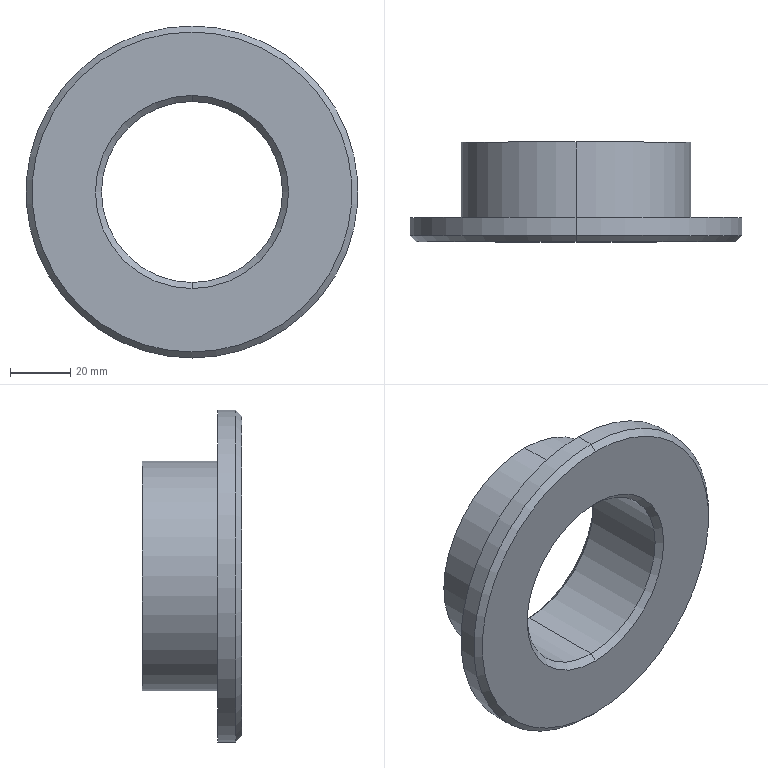Part | SolidWorks | features Chamfer 1, Revolution 1 | 1 solid | 15 faces | box 110 x 33 x 110 mm | volume 94679 mm3 | cone 6 | cylinder 6 | plane 3 | commonest cylinder face diameters 60 x2 76 x2 110 x2
STEP:
#1=CARTESIAN_POINT('',(0.,2.,30.));
#2=VERTEX_POINT('',#1);
#3=CARTESIAN_POINT('',(0.,2.,-30.));
#4=VERTEX_POINT('',#3);
#5=CARTESIAN_POINT('',(0.,2.,0.));
#6=DIRECTION('',(0.,-1.,0.));
#7=DIRECTION('',(0.,0.,1.));
#8=AXIS2_PLACEMENT_3D('',#5,#6,#7);
#9=CIRCLE('',#8,30.);
#10=EDGE_CURVE('',#2,#4,#9,.T.);
#11=ORIENTED_EDGE('',*,*,#10,.F.);
#12=CARTESIAN_POINT('',(0.,0.,32.));
#13=VERTEX_POINT('',#12);
#14=CARTESIAN_POINT('',(0.,2.,30.));
#15=DIRECTION('',(0.,-0.7071,0.7071));
#16=VECTOR('',#15,1000.);
#17=LINE('',#14,#16);
#18=EDGE_CURVE('',#2,#13,#17,.T.);
#19=ORIENTED_EDGE('',*,*,#18,.T.);
#20=CARTESIAN_POINT('',(0.,0.,-32.));
#21=VERTEX_POINT('',#20);
#22=CARTESIAN_POINT('',(0.,0.,0.));
#23=DIRECTION('',(0.,1.,0.));
#24=DIRECTION('',(0.,0.,1.));
#25=AXIS2_PLACEMENT_3D('',#22,#23,#24);
#26=CIRCLE('',#25,32.);
#27=EDGE_CURVE('',#21,#13,#26,.T.);
#28=ORIENTED_EDGE('',*,*,#27,.F.);
#29=CARTESIAN_POINT('',(0.,2.,-30.));
#30=DIRECTION('',(0.,-0.7071,-0.7071));
#31=VECTOR('',#30,1000.);
#32=LINE('',#29,#31);
#33=EDGE_CURVE('',#4,#21,#32,.T.);
#34=ORIENTED_EDGE('',*,*,#33,.F.);
#35=EDGE_LOOP('',(#11,#19,#28,#34));
#36=FACE_OUTER_BOUND('',#35,.T.);
#37=CARTESIAN_POINT('',(0.,2.,0.));
#38=DIRECTION('',(0.,-1.,0.));
#39=DIRECTION('',(0.,0.,-1.));
#40=AXIS2_PLACEMENT_3D('',#37,#38,#39);
#41=CONICAL_SURFACE('',#40,30.,0.7854);
#42=ADVANCED_FACE('',(#36),#41,.F.);
#43=CARTESIAN_POINT('',(0.,31.,-30.));
#44=VERTEX_POINT('',#43);
#45=CARTESIAN_POINT('',(0.,31.,30.));
#46=VERTEX_POINT('',#45);
#47=CARTESIAN_POINT('',(0.,31.,0.));
#48=DIRECTION('',(0.,1.,0.));
#49=DIRECTION('',(0.,0.,-1.));
#50=AXIS2_PLACEMENT_3D('',#47,#48,#49);
#51=CIRCLE('',#50,30.);
#52=EDGE_CURVE('',#44,#46,#51,.T.);
#53=ORIENTED_EDGE('',*,*,#52,.F.);
#54=CARTESIAN_POINT('',(0.,33.,-32.));
#55=VERTEX_POINT('',#54);
#56=CARTESIAN_POINT('',(0.,33.,-32.));
#57=DIRECTION('',(0.,0.7071,-0.7071));
#58=VECTOR('',#57,1000.);
#59=LINE('',#56,#58);
#60=EDGE_CURVE('',#44,#55,#59,.T.);
#61=ORIENTED_EDGE('',*,*,#60,.T.);
#62=CARTESIAN_POINT('',(0.,33.,32.));
#63=VERTEX_POINT('',#62);
#64=CARTESIAN_POINT('',(0.,33.,0.));
#65=DIRECTION('',(0.,-1.,0.));
#66=DIRECTION('',(0.,0.,-1.));
#67=AXIS2_PLACEMENT_3D('',#64,#65,#66);
#68=CIRCLE('',#67,32.);
#69=EDGE_CURVE('',#63,#55,#68,.T.);
#70=ORIENTED_EDGE('',*,*,#69,.F.);
#71=CARTESIAN_POINT('',(0.,33.,32.));
#72=DIRECTION('',(0.,0.7071,0.7071));
#73=VECTOR('',#72,1000.);
#74=LINE('',#71,#73);
#75=EDGE_CURVE('',#46,#63,#74,.T.);
#76=ORIENTED_EDGE('',*,*,#75,.F.);
#77=EDGE_LOOP('',(#53,#61,#70,#76));
#78=FACE_OUTER_BOUND('',#77,.T.);
#79=CARTESIAN_POINT('',(0.,33.,0.));
#80=DIRECTION('',(0.,1.,0.));
#81=DIRECTION('',(0.,0.,1.));
#82=AXIS2_PLACEMENT_3D('',#79,#80,#81);
#83=CONICAL_SURFACE('',#82,32.,0.7854);
#84=ADVANCED_FACE('',(#78),#83,.F.);
#85=CARTESIAN_POINT('',(0.,0.,-53.));
#86=VERTEX_POINT('',#85);
#87=CARTESIAN_POINT('',(0.,0.,53.));
#88=VERTEX_POINT('',#87);
#89=CARTESIAN_POINT('',(0.,0.,0.));
#90=DIRECTION('',(0.,-1.,0.));
#91=DIRECTION('',(0.,0.,1.));
#92=AXIS2_PLACEMENT_3D('',#89,#90,#91);
#93=CIRCLE('',#92,53.);
#94=EDGE_CURVE('',#86,#88,#93,.T.);
#95=ORIENTED_EDGE('',*,*,#94,.F.);
#96=CARTESIAN_POINT('',(0.,2.,-55.));
#97=VERTEX_POINT('',#96);
#98=CARTESIAN_POINT('',(0.,0.,-53.));
#99=DIRECTION('',(0.,0.7071,-0.7071));
#100=VECTOR('',#99,1000.);
#101=LINE('',#98,#100);
#102=EDGE_CURVE('',#86,#97,#101,.T.);
#103=ORIENTED_EDGE('',*,*,#102,.T.);
#104=CARTESIAN_POINT('',(0.,2.,55.));
#105=VERTEX_POINT('',#104);
#106=CARTESIAN_POINT('',(0.,2.,0.));
#107=DIRECTION('',(0.,1.,0.));
#108=DIRECTION('',(0.,0.,1.));
#109=AXIS2_PLACEMENT_3D('',#106,#107,#108);
#110=CIRCLE('',#109,55.);
#111=EDGE_CURVE('',#105,#97,#110,.T.);
#112=ORIENTED_EDGE('',*,*,#111,.F.);
#113=CARTESIAN_POINT('',(0.,0.,53.));
#114=DIRECTION('',(0.,0.7071,0.7071));
#115=VECTOR('',#114,1000.);
#116=LINE('',#113,#115);
#117=EDGE_CURVE('',#88,#105,#116,.T.);
#118=ORIENTED_EDGE('',*,*,#117,.F.);
#119=EDGE_LOOP('',(#95,#103,#112,#118));
#120=FACE_OUTER_BOUND('',#119,.T.);
#121=CARTESIAN_POINT('',(0.,0.,0.));
#122=DIRECTION('',(0.,1.,0.));
#123=DIRECTION('',(0.,0.,1.));
#124=AXIS2_PLACEMENT_3D('',#121,#122,#123);
#125=CONICAL_SURFACE('',#124,53.,0.7854);
#126=ADVANCED_FACE('',(#120),#125,.T.);
#127=CARTESIAN_POINT('',(0.,8.,-55.));
#128=VERTEX_POINT('',#127);
#129=CARTESIAN_POINT('',(0.,8.,55.));
#130=VERTEX_POINT('',#129);
#131=CARTESIAN_POINT('',(0.,8.,0.));
#132=DIRECTION('',(0.,-1.,0.));
#133=DIRECTION('',(0.,0.,-1.));
#134=AXIS2_PLACEMENT_3D('',#131,#132,#133);
#135=CIRCLE('',#134,55.);
#136=EDGE_CURVE('',#128,#130,#135,.T.);
#137=ORIENTED_EDGE('',*,*,#136,.T.);
#138=CARTESIAN_POINT('',(0.,0.,55.));
#139=DIRECTION('',(0.,-1.,0.));
#140=VECTOR('',#139,1000.);
#141=LINE('',#138,#140);
#142=EDGE_CURVE('',#130,#105,#141,.T.);
#143=ORIENTED_EDGE('',*,*,#142,.T.);
#144=ORIENTED_EDGE('',*,*,#111,.T.);
#145=CARTESIAN_POINT('',(0.,0.,-55.));
#146=DIRECTION('',(0.,-1.,0.));
#147=VECTOR('',#146,1000.);
#148=LINE('',#145,#147);
#149=EDGE_CURVE('',#128,#97,#148,.T.);
#150=ORIENTED_EDGE('',*,*,#149,.F.);
#151=EDGE_LOOP('',(#137,#143,#144,#150));
#152=FACE_OUTER_BOUND('',#151,.T.);
#153=CARTESIAN_POINT('',(0.,0.,0.));
#154=DIRECTION('',(0.,-1.,0.));
#155=DIRECTION('',(0.,0.,-1.));
#156=AXIS2_PLACEMENT_3D('',#153,#154,#155);
#157=CYLINDRICAL_SURFACE('',#156,55.);
#158=ADVANCED_FACE('',(#152),#157,.T.);
#159=CARTESIAN_POINT('',(0.,33.,-38.));
#160=VERTEX_POINT('',#159);
#161=CARTESIAN_POINT('',(0.,33.,38.));
#162=VERTEX_POINT('',#161);
#163=CARTESIAN_POINT('',(0.,33.,0.));
#164=DIRECTION('',(0.,-1.,0.));
#165=DIRECTION('',(0.,0.,-1.));
#166=AXIS2_PLACEMENT_3D('',#163,#164,#165);
#167=CIRCLE('',#166,38.);
#168=EDGE_CURVE('',#160,#162,#167,.T.);
#169=ORIENTED_EDGE('',*,*,#168,.T.);
#170=CARTESIAN_POINT('',(0.,8.,38.));
#171=VERTEX_POINT('',#170);
#172=CARTESIAN_POINT('',(0.,0.,38.));
#173=DIRECTION('',(0.,-1.,0.));
#174=VECTOR('',#173,1000.);
#175=LINE('',#172,#174);
#176=EDGE_CURVE('',#162,#171,#175,.T.);
#177=ORIENTED_EDGE('',*,*,#176,.T.);
#178=CARTESIAN_POINT('',(0.,8.,-38.));
#179=VERTEX_POINT('',#178);
#180=CARTESIAN_POINT('',(0.,8.,0.));
#181=DIRECTION('',(0.,-1.,0.));
#182=DIRECTION('',(0.,0.,-1.));
#183=AXIS2_PLACEMENT_3D('',#180,#181,#182);
#184=CIRCLE('',#183,38.);
#185=EDGE_CURVE('',#179,#171,#184,.T.);
#186=ORIENTED_EDGE('',*,*,#185,.F.);
#187=CARTESIAN_POINT('',(0.,0.,-38.));
#188=DIRECTION('',(0.,-1.,0.));
#189=VECTOR('',#188,1000.);
#190=LINE('',#187,#189);
#191=EDGE_CURVE('',#160,#179,#190,.T.);
#192=ORIENTED_EDGE('',*,*,#191,.F.);
#193=EDGE_LOOP('',(#169,#177,#186,#192));
#194=FACE_OUTER_BOUND('',#193,.T.);
#195=CARTESIAN_POINT('',(0.,0.,0.));
#196=DIRECTION('',(0.,-1.,0.));
#197=DIRECTION('',(0.,0.,-1.));
#198=AXIS2_PLACEMENT_3D('',#195,#196,#197);
#199=CYLINDRICAL_SURFACE('',#198,38.);
#200=ADVANCED_FACE('',(#194),#199,.T.);
#201=ORIENTED_EDGE('',*,*,#52,.T.);
#202=CARTESIAN_POINT('',(0.,0.,30.));
#203=DIRECTION('',(0.,-1.,0.));
#204=VECTOR('',#203,1000.);
#205=LINE('',#202,#204);
#206=EDGE_CURVE('',#46,#2,#205,.T.);
#207=ORIENTED_EDGE('',*,*,#206,.T.);
#208=ORIENTED_EDGE('',*,*,#10,.T.);
#209=CARTESIAN_POINT('',(0.,0.,-30.));
#210=DIRECTION('',(0.,-1.,0.));
#211=VECTOR('',#210,1000.);
#212=LINE('',#209,#211);
#213=EDGE_CURVE('',#44,#4,#212,.T.);
#214=ORIENTED_EDGE('',*,*,#213,.F.);
#215=EDGE_LOOP('',(#201,#207,#208,#214));
#216=FACE_OUTER_BOUND('',#215,.T.);
#217=CARTESIAN_POINT('',(0.,0.,0.));
#218=DIRECTION('',(0.,-1.,0.));
#219=DIRECTION('',(0.,0.,-1.));
#220=AXIS2_PLACEMENT_3D('',#217,#218,#219);
#221=CYLINDRICAL_SURFACE('',#220,30.);
#222=ADVANCED_FACE('',(#216),#221,.F.);
#223=CARTESIAN_POINT('',(0.,0.,0.));
#224=DIRECTION('',(0.,-1.,0.));
#225=DIRECTION('',(0.,0.,1.));
#226=AXIS2_PLACEMENT_3D('',#223,#224,#225);
#227=CIRCLE('',#226,53.);
#228=EDGE_CURVE('',#88,#86,#227,.T.);
#229=ORIENTED_EDGE('',*,*,#228,.T.);
#230=ORIENTED_EDGE('',*,*,#94,.T.);
#231=EDGE_LOOP('',(#229,#230));
#232=FACE_OUTER_BOUND('',#231,.T.);
#233=ORIENTED_EDGE('',*,*,#27,.T.);
#234=CARTESIAN_POINT('',(0.,0.,0.));
#235=DIRECTION('',(0.,1.,0.));
#236=DIRECTION('',(0.,0.,1.));
#237=AXIS2_PLACEMENT_3D('',#234,#235,#236);
#238=CIRCLE('',#237,32.);
#239=EDGE_CURVE('',#13,#21,#238,.T.);
#240=ORIENTED_EDGE('',*,*,#239,.T.);
#241=EDGE_LOOP('',(#233,#240));
#242=FACE_BOUND('',#241,.T.);
#243=CARTESIAN_POINT('',(-55.,0.,0.));
#244=DIRECTION('',(0.,1.,0.));
#245=DIRECTION('',(0.,0.,1.));
#246=AXIS2_PLACEMENT_3D('',#243,#244,#245);
#247=PLANE('',#246);
#248=ADVANCED_FACE('',(#232,#242),#247,.F.);
#249=ORIENTED_EDGE('',*,*,#206,.F.);
#250=CARTESIAN_POINT('',(0.,31.,0.));
#251=DIRECTION('',(0.,1.,0.));
#252=DIRECTION('',(0.,0.,-1.));
#253=AXIS2_PLACEMENT_3D('',#250,#251,#252);
#254=CIRCLE('',#253,30.);
#255=EDGE_CURVE('',#46,#44,#254,.T.);
#256=ORIENTED_EDGE('',*,*,#255,.T.);
#257=ORIENTED_EDGE('',*,*,#213,.T.);
#258=CARTESIAN_POINT('',(0.,2.,0.));
#259=DIRECTION('',(0.,-1.,0.));
#260=DIRECTION('',(0.,0.,1.));
#261=AXIS2_PLACEMENT_3D('',#258,#259,#260);
#262=CIRCLE('',#261,30.);
#263=EDGE_CURVE('',#4,#2,#262,.T.);
#264=ORIENTED_EDGE('',*,*,#263,.T.);
#265=EDGE_LOOP('',(#249,#256,#257,#264));
#266=FACE_OUTER_BOUND('',#265,.T.);
#267=CARTESIAN_POINT('',(0.,0.,0.));
#268=DIRECTION('',(0.,-1.,0.));
#269=DIRECTION('',(0.,0.,-1.));
#270=AXIS2_PLACEMENT_3D('',#267,#268,#269);
#271=CYLINDRICAL_SURFACE('',#270,30.);
#272=ADVANCED_FACE('',(#266),#271,.F.);
#273=ORIENTED_EDGE('',*,*,#69,.T.);
#274=CARTESIAN_POINT('',(0.,33.,0.));
#275=DIRECTION('',(0.,-1.,0.));
#276=DIRECTION('',(0.,0.,-1.));
#277=AXIS2_PLACEMENT_3D('',#274,#275,#276);
#278=CIRCLE('',#277,32.);
#279=EDGE_CURVE('',#55,#63,#278,.T.);
#280=ORIENTED_EDGE('',*,*,#279,.T.);
#281=EDGE_LOOP('',(#273,#280));
#282=FACE_BOUND('',#281,.T.);
#283=ORIENTED_EDGE('',*,*,#168,.F.);
#284=CARTESIAN_POINT('',(0.,33.,0.));
#285=DIRECTION('',(0.,-1.,0.));
#286=DIRECTION('',(0.,0.,-1.));
#287=AXIS2_PLACEMENT_3D('',#284,#285,#286);
#288=CIRCLE('',#287,38.);
#289=EDGE_CURVE('',#162,#160,#288,.T.);
#290=ORIENTED_EDGE('',*,*,#289,.F.);
#291=EDGE_LOOP('',(#283,#290));
#292=FACE_OUTER_BOUND('',#291,.T.);
#293=CARTESIAN_POINT('',(-30.,33.,0.));
#294=DIRECTION('',(0.,-1.,0.));
#295=DIRECTION('',(0.,0.,-1.));
#296=AXIS2_PLACEMENT_3D('',#293,#294,#295);
#297=PLANE('',#296);
#298=ADVANCED_FACE('',(#282,#292),#297,.F.);
#299=ORIENTED_EDGE('',*,*,#176,.F.);
#300=ORIENTED_EDGE('',*,*,#289,.T.);
#301=ORIENTED_EDGE('',*,*,#191,.T.);
#302=CARTESIAN_POINT('',(0.,8.,0.));
#303=DIRECTION('',(0.,-1.,0.));
#304=DIRECTION('',(0.,0.,-1.));
#305=AXIS2_PLACEMENT_3D('',#302,#303,#304);
#306=CIRCLE('',#305,38.);
#307=EDGE_CURVE('',#171,#179,#306,.T.);
#308=ORIENTED_EDGE('',*,*,#307,.F.);
#309=EDGE_LOOP('',(#299,#300,#301,#308));
#310=FACE_OUTER_BOUND('',#309,.T.);
#311=CARTESIAN_POINT('',(0.,0.,0.));
#312=DIRECTION('',(0.,-1.,0.));
#313=DIRECTION('',(0.,0.,-1.));
#314=AXIS2_PLACEMENT_3D('',#311,#312,#313);
#315=CYLINDRICAL_SURFACE('',#314,38.);
#316=ADVANCED_FACE('',(#310),#315,.T.);
#317=ORIENTED_EDGE('',*,*,#136,.F.);
#318=CARTESIAN_POINT('',(0.,8.,0.));
#319=DIRECTION('',(0.,-1.,0.));
#320=DIRECTION('',(0.,0.,-1.));
#321=AXIS2_PLACEMENT_3D('',#318,#319,#320);
#322=CIRCLE('',#321,55.);
#323=EDGE_CURVE('',#130,#128,#322,.T.);
#324=ORIENTED_EDGE('',*,*,#323,.F.);
#325=EDGE_LOOP('',(#317,#324));
#326=FACE_OUTER_BOUND('',#325,.T.);
#327=ORIENTED_EDGE('',*,*,#185,.T.);
#328=ORIENTED_EDGE('',*,*,#307,.T.);
#329=EDGE_LOOP('',(#327,#328));
#330=FACE_BOUND('',#329,.T.);
#331=CARTESIAN_POINT('',(-38.,8.,0.));
#332=DIRECTION('',(0.,-1.,0.));
#333=DIRECTION('',(0.,0.,-1.));
#334=AXIS2_PLACEMENT_3D('',#331,#332,#333);
#335=PLANE('',#334);
#336=ADVANCED_FACE('',(#326,#330),#335,.F.);
#337=ORIENTED_EDGE('',*,*,#142,.F.);
#338=ORIENTED_EDGE('',*,*,#323,.T.);
#339=ORIENTED_EDGE('',*,*,#149,.T.);
#340=CARTESIAN_POINT('',(0.,2.,0.));
#341=DIRECTION('',(0.,1.,0.));
#342=DIRECTION('',(0.,0.,1.));
#343=AXIS2_PLACEMENT_3D('',#340,#341,#342);
#344=CIRCLE('',#343,55.);
#345=EDGE_CURVE('',#97,#105,#344,.T.);
#346=ORIENTED_EDGE('',*,*,#345,.T.);
#347=EDGE_LOOP('',(#337,#338,#339,#346));
#348=FACE_OUTER_BOUND('',#347,.T.);
#349=CARTESIAN_POINT('',(0.,0.,0.));
#350=DIRECTION('',(0.,-1.,0.));
#351=DIRECTION('',(0.,0.,-1.));
#352=AXIS2_PLACEMENT_3D('',#349,#350,#351);
#353=CYLINDRICAL_SURFACE('',#352,55.);
#354=ADVANCED_FACE('',(#348),#353,.T.);
#355=ORIENTED_EDGE('',*,*,#102,.F.);
#356=ORIENTED_EDGE('',*,*,#228,.F.);
#357=ORIENTED_EDGE('',*,*,#117,.T.);
#358=ORIENTED_EDGE('',*,*,#345,.F.);
#359=EDGE_LOOP('',(#355,#356,#357,#358));
#360=FACE_OUTER_BOUND('',#359,.T.);
#361=CARTESIAN_POINT('',(0.,0.,0.));
#362=DIRECTION('',(0.,1.,0.));
#363=DIRECTION('',(0.,0.,1.));
#364=AXIS2_PLACEMENT_3D('',#361,#362,#363);
#365=CONICAL_SURFACE('',#364,53.,0.7854);
#366=ADVANCED_FACE('',(#360),#365,.T.);
#367=ORIENTED_EDGE('',*,*,#60,.F.);
#368=ORIENTED_EDGE('',*,*,#255,.F.);
#369=ORIENTED_EDGE('',*,*,#75,.T.);
#370=ORIENTED_EDGE('',*,*,#279,.F.);
#371=EDGE_LOOP('',(#367,#368,#369,#370));
#372=FACE_OUTER_BOUND('',#371,.T.);
#373=CARTESIAN_POINT('',(0.,33.,0.));
#374=DIRECTION('',(0.,1.,0.));
#375=DIRECTION('',(0.,0.,1.));
#376=AXIS2_PLACEMENT_3D('',#373,#374,#375);
#377=CONICAL_SURFACE('',#376,32.,0.7854);
#378=ADVANCED_FACE('',(#372),#377,.F.);
#379=ORIENTED_EDGE('',*,*,#18,.F.);
#380=ORIENTED_EDGE('',*,*,#263,.F.);
#381=ORIENTED_EDGE('',*,*,#33,.T.);
#382=ORIENTED_EDGE('',*,*,#239,.F.);
#383=EDGE_LOOP('',(#379,#380,#381,#382));
#384=FACE_OUTER_BOUND('',#383,.T.);
#385=CARTESIAN_POINT('',(0.,2.,0.));
#386=DIRECTION('',(0.,-1.,0.));
#387=DIRECTION('',(0.,0.,-1.));
#388=AXIS2_PLACEMENT_3D('',#385,#386,#387);
#389=CONICAL_SURFACE('',#388,30.,0.7854);
#390=ADVANCED_FACE('',(#384),#389,.F.);
#391=CLOSED_SHELL('',(#42,#84,#126,#158,#200,#222,#248,#272,#298,#316,#336,#354,#366,#378,#390));
#392=MANIFOLD_SOLID_BREP('',#391);
#393=CARTESIAN_POINT('',(0.,0.,0.));
#394=DIRECTION('',(0.,0.,1.));
#395=DIRECTION('',(1.,0.,0.));
#396=AXIS2_PLACEMENT_3D('',#393,#394,#395);
#397=(LENGTH_UNIT()NAMED_UNIT(*)SI_UNIT(.MILLI.,.METRE.));
#398=UNCERTAINTY_MEASURE_WITH_UNIT(LENGTH_MEASURE(0.00001),#397,'','');
#399=(NAMED_UNIT(*)PLANE_ANGLE_UNIT()SI_UNIT($,.RADIAN.));
#400=(NAMED_UNIT(*)SI_UNIT($,.STERADIAN.)SOLID_ANGLE_UNIT());
#401=(GEOMETRIC_REPRESENTATION_CONTEXT(3)GLOBAL_UNCERTAINTY_ASSIGNED_CONTEXT((#398))GLOBAL_UNIT_ASSIGNED_CONTEXT((#397,#399,#400))REPRESENTATION_CONTEXT('',''));
#402=ADVANCED_BREP_SHAPE_REPRESENTATION('',(#392,#396),#401);